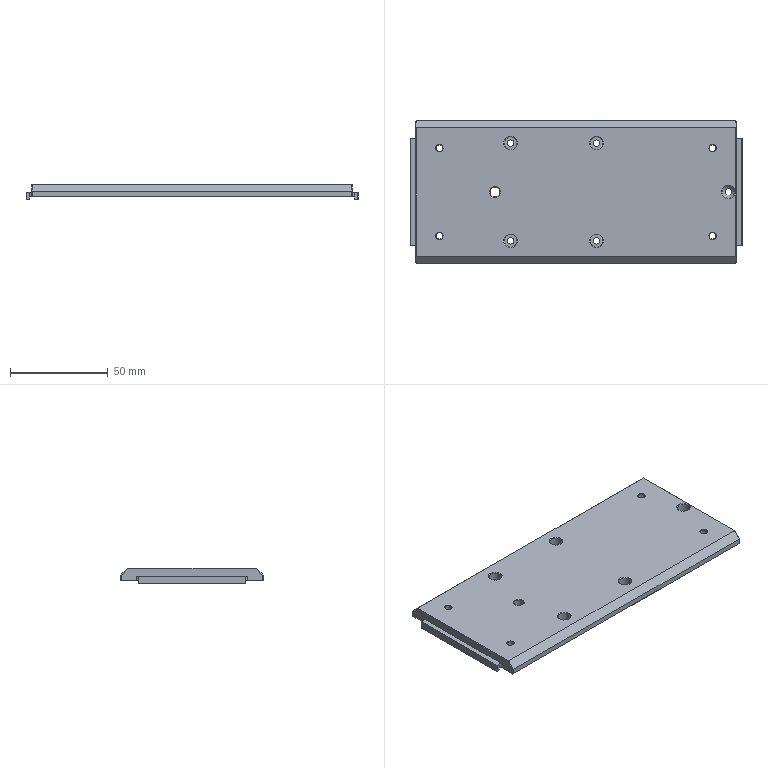Part | SolidWorks | features BaseBody 1 | 1 solid | 112 faces | box 170 x 73 x 8 mm | volume 75730 mm3 | plane 54 | cylinder 34 | cone 24 | commonest cylinder face diameters 3.4 x10 6.4 x10 3.3 x8 2 x4 5 x2